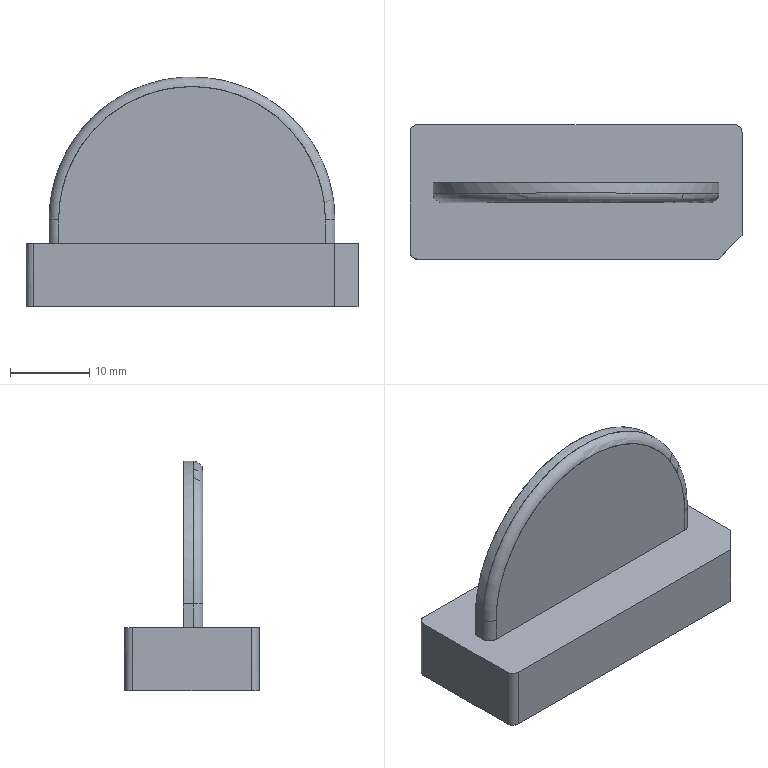NC program | PowerMill | posted with a generic post | part box 42 x 17 x 29.081 mm
Lines 1 to 998 of 145628:
%
O0001
N104 ( POWERMILL CB  : 2026004.0)
N105 ( POST VER      : 2026.0.0.5161)
N106 ( OPTION FILE   : FANUC)
N107 ( OUTPUT WORKPLANE : WORLD)
N108 (  )
N109 ( TOOL LIST )
N110 (---------------------------------------)
N111 ( NO. | ID        | DIA.| TIP RAD|LENGTH)
N112 (---------------------------------------)
N113 (    1|D10C_1_1_1 |10.0 |  0.0   |84.52 )
N114 (    2|D4C_1_1    | 4.0 |  0.0   |76.08 )
N115 (    3|D10_1_1_1  |10.0 |  0.0   |84.24 )
N116 (    7|R2_1_1     | 4.0 |  2.0   | 75.4 )
N117 (   14|D4_1_1     | 4.0 |  0.0   |76.36 )
N118 (   13|TEXT_D4_1_1| 4.0 |  0.3   |76.36 )
N119 (---------------------------------------)
N120 (  )
N121 ( NUMBER OF TOOLPATHS: 10.0 )
N122 ( ESTIMATED PROGRAM DURATION: 0 HOURS 22 MIN 21 SEC)
N123 (  )
N124 G00 G21 G80 G40 G17
N125 G90
N126 G54
N127 G53 Z0.0
N128 (---------------)
N129 ( START TOOLPATH : 精公开粗01-扫面平行-D10C )
N130 (---------------)
N131 ( TOOL NO.    :1 )
N132 ( TOOL TYPE   : ENDMILL)
N133 ( TOOL ID     : D10C_1_1_1)
N134 ( TOOL DIA    : 10.0 LENGTH 84.52)
N135 T1
N136 M6
N137 S8000 M03
N138 G00 G90 X0.0 Y0.0
N139 G43 Z10.2 H1
N140
N141 G05 P10000 R4
N142 X28.78 Y11.28
N143 Z1.128
N144 G01 Z-0.072 F6000.0
N145 X23.78 F10000.0
N146 X-23.78
N147 Y5.64
N148 X23.78
N149 Y0.0
N150 X-23.78
N151 Y-5.64
N152 X23.78
N153 Y-11.28
N154 X-23.78
N155 X-28.78
N156 G00 Z10.2
N157 G05 P0
N158 (---------------)
N159 ( END TOOLPATH : 精公开粗01-扫面平行-D10C )
N160 (---------------)
N161 ( START TOOLPATH : 精公开粗01-外形偏置-D10C )
N162 (---------------)
N163 G00 X-0.0005 Y0.0 Z9.878
N164 G05 P10000 R4
N165 X-4.748 Y16.555
N166 Z0.6824
N167 G01 Z-0.5176 F6000.0
N168 Y16.0275 F10000.0
N169 G03 X-0.0005 Y11.28 I4.7475 J0.0
N170 G01 X24.86
N171 G02 X25.86 Y10.28 I0.0 J-1.0
N172 G01 Y-10.28
N173 G02 X24.86 Y-11.28 I-1.0 J0.0
N174 G01 X-24.861
N175 G02 X-25.861 Y-10.28 I0.0 J1.0
N176 G01 Y10.28
N177 G02 X-24.861 Y11.28 I1.0 J0.0
N178 G01 X-0.0005
N179 Y6.4169
N180 X3.0932 Y6.4168
N181 X3.8666 Y6.399
N182 X4.6401 Y6.3013
N183 X5.4135 Y6.092
N184 X6.0959 Y5.8007
N185 X6.9603 Y5.248
N186 X7.2226 Y5.0273
N187 X7.7338 Y4.5003
N188 X7.9275 Y4.2538
N189 X8.4055 Y3.4804
N190 X8.7187 Y2.707
N191 X8.8992 Y1.9336
N192 X8.9604 Y1.1601
N193 X8.9637 Y-0.3867
N194 X8.9175 Y-0.7813
N195 X14.4064 Y-1.5077
N196 X14.4426 Y-1.2341
N197 G03 X14.5447 Y0.9936 I-12.9021 J1.7075
N198 G01 X14.4426 Y3.5466
N199 G02 X16.748 Y5.6029 I1.9984 J0.08
N200 G01 X18.2762 Y5.3655
N201 G02 X19.9692 Y3.3892 I-0.307 J-1.9763
N202 G01 Y-3.3892
N203 G02 X18.2883 Y-5.3636 I-2.0 J0.0
N204 G01 X16.4548 Y-5.6599
N205 G02 X14.1529 Y-3.4232 I-0.3192 J1.9743
N206 G01 X14.4064 Y-1.5077
N207 X8.9175 Y-0.7813
N208 X8.8732 Y-1.1601
N209 X8.6608 Y-1.9336
N210 X8.3269 Y-2.707
N211 X7.8601 Y-3.4804
N212 X7.7338 Y-3.6456
N213 X7.1694 Y-4.2538
N214 X6.9603 Y-4.4341
N215 X6.1869 Y-4.9724
N216 X5.4135 Y-5.3841
N217 X4.2469 Y-5.8007
N218 X3.8666 Y-5.9112
N219 X3.0932 Y-6.0572
N220 X2.3198 Y-6.1645
N221 X0.7729 Y-6.2839
N222 X-0.7739 Y-6.2838
N223 X-2.3208 Y-6.1644
N224 X-3.0942 Y-6.0571
N225 X-3.8676 Y-5.911
N226 X-4.2415 Y-5.8007
N227 X-5.4145 Y-5.3836
N228 X-6.0923 Y-5.0273
N229 X-6.9613 Y-4.4332
N230 X-7.1687 Y-4.2538
N231 X-7.7348 Y-3.6443
N232 X-7.8604 Y-3.4804
N233 X-8.3275 Y-2.707
N234 X-8.6608 Y-1.9336
N235 X-8.8732 Y-1.1601
N236 X-8.8858 Y-1.0529
N237 X-14.3677 Y-1.7757
N238 X-14.1505 Y-3.4225
N239 G02 X-16.4503 Y-5.6587 I-1.9829 J-0.2614
N240 G01 X-18.2871 Y-5.3639
N241 G02 X-19.9702 Y-3.3892 I0.3169 J1.9747
N242 G01 Y3.3892
N243 G02 X-18.3054 Y5.3609 I2.0 J0.0
N244 G01 X-16.8126 Y5.6146
N245 G02 X-14.4781 Y3.5924 I0.3351 J-1.9717
N246 G01 X-14.5483 Y0.8173
N247 G03 X-14.44 Y-1.2268 I13.0978 J-0.3313
N248 G01 X-14.3677 Y-1.7757
N249 X-8.8858 Y-1.0529
N250 X-8.9637 Y-0.3867
N251 X-8.9611 Y1.1601
N252 X-8.9 Y1.9336
N253 X-8.7217 Y2.707
N254 X-8.4055 Y3.4804
N255 X-7.9294 Y4.2538
N256 X-7.7348 Y4.4991
N257 X-7.2239 Y5.0273
N258 X-6.9613 Y5.2472
N259 X-6.1879 Y5.7527
N260 X-5.4145 Y6.0917
N261 X-4.6411 Y6.3012
N262 X-3.8676 Y6.3989
N263 X-3.0942 Y6.4169
N264 X-0.0005
N265 Y11.28
N266 G00 Z3.2868
N267 G01 X-4.748 Y16.555
N268 G00 Z0.2868
N269 G01 Z-0.9132 F6000.0
N270 Y16.0275 F10000.0
N271 G03 X-0.0005 Y11.28 I4.7475 J0.0
N272 G01 X24.86
N273 G02 X25.86 Y10.28 I0.0 J-1.0
N274 G01 Y-10.28
N275 G02 X24.86 Y-11.28 I-1.0 J0.0
N276 G01 X1.6308
N277 X1.5464 Y-6.5239
N278 X-0.0005 Y-6.5514
N279 X-1.5474 Y-6.5239
N280 X-3.0942 Y-6.4283
N281 X-4.6411 Y-6.2118
N282 X-5.4145 Y-6.0286
N283 X-6.1879 Y-5.8046
N284 X-6.9613 Y-5.4754
N285 X-7.7663 Y-5.0273
N286 X-8.5082 Y-4.4458
N287 X-8.7163 Y-4.2538
N288 X-9.4061 Y-3.4804
N289 X-9.8711 Y-2.707
N290 X-10.1967 Y-1.9336
N291 X-10.3646 Y-1.3222
N292 X-15.8819 Y-2.0602
N293 X-15.6998 Y-3.4218
N294 G02 X-19.1197 Y-5.0774 I-1.9824 J-0.2651
N295 G01 X-19.4077 Y-4.7797
N296 G02 X-19.9702 Y-3.3949 I1.4375 J1.3905
N297 G01 X-19.9901 Y3.6217
N298 G02 X-17.9524 Y5.6271 I2.0 J0.0057
N299 G02 X-15.9917 Y3.5464 I-0.0377 J-1.9997
N300 G01 X-16.095 Y1.0006
N301 G03 X-15.9912 Y-1.2433 I12.9526 J-0.5253
N302 G01 X-15.8819 Y-2.0602
N303 X-10.3646 Y-1.3222
N304 X-10.4092 Y-1.1601
N305 X-10.4958 Y-0.3867
N306 X-10.4842 Y0.3867
N307 X-10.5041 Y1.1601
N308 X-10.4473 Y1.9336
N309 X-10.2658 Y2.707
N310 X-9.954 Y3.4804
N311 X-9.4782 Y4.2538
N312 X-9.2816 Y4.5006
N313 X-8.7737 Y5.0273
N314 X-8.5082 Y5.2463
N315 X-7.7348 Y5.7549
N316 X-6.9613 Y6.0949
N317 X-6.1879 Y6.3042
N318 X-5.4145 Y6.4037
N319 X-4.6411 Y6.4168
N320 X-3.0953
N321 X-3.0942
N322 X-0.454
N323 X4.6401
N324 X5.4135 Y6.4037
N325 X6.1869 Y6.3042
N326 X6.9603 Y6.0953
N327 X7.6483 Y5.8007
N328 X8.5072 Y5.2471
N329 X8.7731 Y5.0273
N330 X9.2806 Y4.5022
N331 X9.4777 Y4.2538
N332 X9.9534 Y3.4804
N333 X10.268 Y2.707
N334 X10.4355 Y1.9892
N335 X16.0291 Y2.2327
N336 X15.9727 Y3.5286
N337 G02 X17.9275 Y5.6152 I1.9981 J0.0871
N338 G02 X19.9708 Y3.6152 I0.0433 J-1.9995
N339 G01 X19.9692 Y-3.3896
N340 G02 X19.426 Y-4.7594 I-2.0 J0.0004
N341 G01 X19.1441 Y-5.0592
N342 G02 X15.7045 Y-3.4271 I-1.4568 J1.3703
N343 G01 X15.9883 Y-1.2779
N344 G03 X16.0856 Y0.9368 I-12.5877 J1.6623
N345 G01 X16.0291 Y2.2327
N346 X10.4355 Y1.9892
N347 X10.4485 Y1.9336
N348 X10.5096 Y1.1601
N349 X10.4844 Y0.3867
N350 X10.4846 Y0.3741
N351 X10.4984 Y-0.3867
N352 X10.4091 Y-1.1601
N353 X10.1957 Y-1.9336
N354 X9.8723 Y-2.707
N355 X9.4032 Y-3.4804
N356 X8.7151 Y-4.2538
N357 X8.5072 Y-4.4467
N358 X7.7661 Y-5.0273
N359 X6.9603 Y-5.4759
N360 X6.2009 Y-5.8007
N361 X5.4135 Y-6.0289
N362 X4.6401 Y-6.212
N363 X3.0932 Y-6.4283
N364 X1.5464 Y-6.5239
N365 X1.6308 Y-11.28
N366 X-24.861
N367 G02 X-25.861 Y-10.28 I0.0 J1.0
N368 G01 Y10.28
N369 G02 X-24.861 Y11.28 I1.0 J0.0
N370 G01 X-0.0005
N371 G00 Z2.8911
N372 G01 X-4.748 Y16.555
N373 G00 Z-0.1089
N374 G01 Z-1.3089 F6000.0
N375 Y16.0275 F10000.0
N376 G03 X-0.0005 Y11.28 I4.7475 J0.0
N377 G01 X24.86
N378 G02 X25.86 Y10.28 I0.0 J-1.0
N379 G01 Y-0.0376
N380 X20.276 Y0.0037
N381 X20.2473 Y-3.8741
N382 G02 X18.4916 Y-5.5316 I-1.6719 J0.0124
N383 G02 X16.9106 Y-3.7066 I0.0838 J1.6699
N384 G01 X17.1834 Y-0.7784
N385 G03 X17.1729 Y1.8028 I-13.2777 J1.2368
N386 G01 X16.9842 Y3.6645
N387 G02 X17.6255 Y4.9931 I1.4025 J0.1422
N388 G01 X17.932 Y5.1897
N389 G02 X20.3047 Y3.8814 I0.8319 J-1.2969
N390 G01 X20.276 Y0.0037
N391 X25.86 Y-0.0376
N392 Y-10.28
N393 G02 X24.86 Y-11.28 I-1.0 J0.0
N394 G01 X1.9457
N395 X1.7958 Y-6.6304
N396 X1.5464 Y-6.6384
N397 X-2.3208 Y-6.6259
N398 X-3.8676 Y-6.5553
N399 X-5.4145 Y-6.3754
N400 X-6.1879 Y-6.2106
N401 X-6.9613 Y-6.0057
N402 X-7.5259 Y-5.8007
N403 X-8.5082 Y-5.3279
N404 X-9.2816 Y-4.8217
N405 X-9.9246 Y-4.2538
N406 X-10.5863 Y-3.4804
N407 X-10.8285 Y-3.1157
N408 X-11.0524 Y-2.707
N409 X-11.3596 Y-1.9336
N410 X-11.57 Y-1.1601
N411 X-11.6598 Y-0.3867
N412 X-11.6619 Y1.1601
N413 X-11.6006 Y1.9336
N414 X-11.4218 Y2.707
N415 X-11.1075 Y3.4804
N416 X-10.8285 Y3.972
N417 X-10.632 Y4.2538
N418 X-10.055 Y4.9096
N419 X-9.2816 Y5.5284
N420 X-8.8142 Y5.8007
N421 X-8.5082 Y5.9471
N422 X-7.7348 Y6.2184
N423 X-6.9613 Y6.3703
N424 X-6.1879 Y6.4168
N425 X6.1869
N426 X6.9603 Y6.3705
N427 X7.7338 Y6.2193
N428 X8.5072 Y5.9476
N429 X8.8128 Y5.8007
N430 X9.2806 Y5.5277
N431 X9.9301 Y5.0273
N432 X10.632 Y4.2538
N433 X10.8275 Y3.9723
N434 X11.1072 Y3.4804
N435 X11.4211 Y2.707
N436 X11.6013 Y1.9336
N437 X11.6624 Y1.1601
N438 X11.6595 Y-0.3867
N439 X11.5703 Y-1.1601
N440 X11.3589 Y-1.9336
N441 X11.0524 Y-2.707
N442 X10.8275 Y-3.1176
N443 X10.5863 Y-3.4804
N444 X9.9243 Y-4.2538
N445 X9.2806 Y-4.8225
N446 X8.5072 Y-5.3285
N447 X7.7338 Y-5.7153
N448 X6.9603 Y-6.006
N449 X6.1869 Y-6.2108
N450 X5.4135 Y-6.3756
N451 X4.6401 Y-6.4769
N452 X3.5423 Y-6.5741
N453 X1.7958 Y-6.6304
N454 X1.9457 Y-11.28
N455 X-24.861
N456 G02 X-25.861 Y-10.28 I0.0 J1.0
N457 G01 Y-0.0375
N458 X-20.2862 Y0.0035
N459 X-20.3147 Y3.8862
N460 G02 X-17.945 Y5.1964 I1.5407 J0.0114
N461 G01 X-17.6293 Y4.9949
N462 G02 X-16.987 Y3.648 I-0.7584 J-1.1882
N463 G01 X-17.1834 Y1.9149
N464 G03 X-17.0637 Y-1.8414 I12.9517 J-1.4676
N465 G01 X-16.778 Y-3.4433
N466 G02 X-17.0925 Y-4.6773 I-1.5169 J-0.2706
N467 G01 X-17.2809 Y-4.9125
N468 G02 X-20.2576 Y-3.8793 I-1.3048 J1.0455
N469 G01 X-20.2862 Y0.0035
N470 X-25.861 Y-0.0375
N471 Y10.28
N472 G02 X-24.861 Y11.28 I1.0 J0.0
N473 G01 X-0.0005
N474 G00 Z2.4955
N475 G01 X-4.748 Y16.555
N476 G00 Z-0.5045
N477 G01 Z-1.7045 F6000.0
N478 Y16.0275 F10000.0
N479 G03 X-0.0005 Y11.28 I4.7475 J0.0
N480 G01 X24.86
N481 G02 X25.86 Y10.28 I0.0 J-1.0
N482 G01 Y-10.28
N483 G02 X24.86 Y-11.28 I-1.0 J0.0
N484 G01 X4.171
N485 X4.06 Y-6.6312
N486 X3.0932 Y-6.6543
N487 X-3.0942
N488 X-4.6411 Y-6.6173
N489 X-5.4145 Y-6.5549
N490 X-6.1879 Y-6.4616
N491 X-6.9613 Y-6.3203
N492 X-7.7348 Y-6.1167
N493 X-8.5082 Y-5.8507
N494 X-9.2816 Y-5.4811
N495 X-9.9973 Y-5.0273
N496 X-10.8285 Y-4.3444
N497 X-11.5537 Y-3.4804
N498 X-12.0192 Y-2.707
N499 X-12.3227 Y-1.9336
N500 X-12.5179 Y-1.1601
N501 X-12.6081 Y-0.3867
N502 X-12.5915 Y0.3867
N503 X-12.6157 Y1.1601
N504 X-12.5592 Y1.878
N505 X-17.9775 Y2.9102
N506 G03 X-17.8345 Y-2.6932 I12.9773 J-2.4723
N507 G01 X-17.5688 Y-3.7822
N508 G02 X-18.2144 Y-5.0414 I-1.0508 J-0.2564
N509 G01 X-18.6701 Y-5.2256
N510 G02 X-20.2471 Y-4.1712 I-0.4298 J1.0637
N511 G01 X-20.3147 Y4.1962
N512 G02 X-19.0619 Y5.1925 I1.0159 J0.0083
N513 G01 X-18.4908 Y5.0556
N514 G02 X-17.7788 Y3.9535 I-0.2216 J-0.9242
N515 G01 X-17.9775 Y2.9102
N516 X-12.5592 Y1.878
N517 X-12.5548 Y1.9336
N518 X-12.3746 Y2.707
N519 X-12.0616 Y3.4804
N520 X-11.5864 Y4.2538
N521 X-10.8845 Y5.0273
N522 X-10.055 Y5.6404
N523 X-9.7687 Y5.8007
N524 X-9.2816 Y6.0228
N525 X-8.5082 Y6.2663
N526 X-7.7348 Y6.391
N527 X-6.9613 Y6.4169
N528 X6.9603
N529 X7.7338 Y6.3911
N530 X8.5072 Y6.2666
N531 X9.2806 Y6.0234
N532 X9.7687 Y5.8007
N533 X10.054 Y5.641
N534 X10.8275 Y5.0755
N535 X11.5864 Y4.2538
N536 X12.0616 Y3.4804
N537 X12.3746 Y2.707
N538 X12.4755 Y2.2737
N539 X17.9038 Y3.2589
N540 X17.7762 Y3.9616
N541 G02 X18.4913 Y5.0559 I0.9352 J0.1698
N542 G01 X19.0586 Y5.191
N543 G02 X20.3098 Y4.1956 I0.2353 J-0.9884
N544 G01 X20.2525 Y-4.1637
N545 G02 X18.6929 Y-5.2263 I-1.1472 J0.0079
N546 G01 X18.2298 Y-5.0479
N547 G02 X17.5655 Y-3.7917 I0.3888 J1.0093
N548 G01 X17.842 Y-2.6127
N549 G03 X17.9803 Y2.8372 I-13.0422 J3.0578
N550 G01 X17.9038 Y3.2589
N551 X12.4755 Y2.2737
N552 X12.5548 Y1.9336
N553 X12.6157 Y1.1601
N554 X12.5914 Y0.3867
N555 X12.5917 Y0.3735
N556 X12.6081 Y-0.3867
N557 X12.5179 Y-1.1601
N558 X12.3246 Y-1.9336
N559 X12.0192 Y-2.707
N560 X11.6009 Y-3.4099
N561 X10.9186 Y-4.2538
N562 X10.054 Y-4.9862
N563 X9.2806 Y-5.4817
N564 X8.6222 Y-5.8007
N565 X7.7338 Y-6.117
N566 X6.9603 Y-6.3205
N567 X6.1869 Y-6.4618
N568 X5.1898 Y-6.5741
N569 X4.6401 Y-6.6174
N570 X4.06 Y-6.6312
N571 X4.171 Y-11.28
N572 X-24.861
N573 G02 X-25.861 Y-10.28 I0.0 J1.0
N574 G01 Y10.28
N575 G02 X-24.861 Y11.28 I1.0 J0.0
N576 G01 X-0.0005
N577 G00 Z2.0999
N578 G01 X-4.748 Y16.555
N579 G00 Z-0.9001
N580 G01 Z-2.1001 F6000.0
N581 Y16.0275 F10000.0
N582 G03 X-0.0005 Y11.28 I4.7475 J0.0
N583 G01 X24.86
N584 G02 X25.86 Y10.28 I0.0 J-1.0
N585 G01 Y-10.28
N586 G02 X24.86 Y-11.28 I-1.0 J0.0
N587 G01 X5.0071
N588 X4.8334 Y-6.647
N589 X4.6401 Y-6.6543
N590 X-4.6411
N591 X-6.1879 Y-6.5962
N592 X-6.9613 Y-6.5145
N593 X-7.7348 Y-6.3715
N594 X-8.5082 Y-6.1769
N595 X-9.2816 Y-5.9168
N596 X-10.055 Y-5.545
N597 X-10.8864 Y-5.0273
N598 X-11.7725 Y-4.2538
N599 X-12.3753 Y-3.4949
N600 X-12.8498 Y-2.707
N601 X-13.155 Y-1.9336
N602 X-13.3428 Y-1.1601
N603 X-13.4339 Y-0.3867
N604 X-13.4319 Y1.1601
N605 X-13.3703 Y1.9336
N606 X-13.1917 Y2.707
N607 X-12.8775 Y3.4804
N608 X-12.403 Y4.2538
N609 X-11.7023 Y5.0273
N610 X-10.8285 Y5.6672
N611 X-10.5893 Y5.8007
N612 X-10.055 Y6.0427
N613 X-9.2816 Y6.279
N614 X-8.5082 Y6.3978
N615 X-7.7348 Y6.4169
N616 X7.7338 Y6.4168
N617 X8.5072 Y6.3979
N618 X9.2806 Y6.2782
N619 X10.054 Y6.0419
N620 X10.5896 Y5.8007
N621 X10.8275 Y5.668
N622 X11.6009 Y5.1148
N623 X12.3743 Y4.292
N624 X12.8775 Y3.4804
N625 X13.1477 Y2.8321
N626 X13.3209 Y2.1326
N627 X19.0523 Y3.2808
N628 X18.7789 Y4.6456
N629 G02 X19.3181 Y5.3716 I0.5973 J0.1197
N630 G02 X19.9853 Y4.7611 I0.0581 J-0.6063
N631 G01 X19.9221 Y-4.5604
N632 X19.9147 Y-4.6628
N633 X19.8941 Y-4.7635
N634 X19.8548 Y-4.9063
N635 G02 X18.9354 Y-5.4138 I-0.7069 J0.1942
N636 G02 X18.452 Y-4.4815 I0.2125 J0.7016
N637 G01 X18.6616 Y-3.8491
N638 G03 X19.2578 Y-0.7416 I-11.5446 J3.8261
N639 G01 X19.2667 Y-0.5927
N640 X19.2905 Y0.075
N641 X19.2829 Y0.7432
N642 X19.255 Y1.5452
N643 G03 X19.0523 Y3.2808 I-10.7315 J-0.3736
N644 G01 X13.3209 Y2.1326
N645 X13.3702 Y1.9336
N646 X13.4311 Y1.1601
N647 X13.4356 Y-0.3867
N648 X13.3455 Y-1.1601
N649 X13.1538 Y-1.9336
N650 X12.8498 Y-2.707
N651 X12.3866 Y-3.4804
N652 X11.7732 Y-4.2538
N653 X10.8863 Y-5.0273
N654 X10.054 Y-5.5455
N655 X9.5583 Y-5.8007
N656 X9.2806 Y-5.9172
N657 X8.5072 Y-6.1773
N658 X7.7338 Y-6.3717
N659 X6.9603 Y-6.5147
N660 X6.4087 Y-6.5741
N661 X6.1869 Y-6.5963
N662 X4.8334 Y-6.647
N663 X5.0071 Y-11.28
N664 X-24.861
N665 G02 X-25.861 Y-10.28 I0.0 J1.0
N666 G01 Y-0.0035
N667 X-19.9717 Y0.0617
N668 X-20.0235 Y4.7512
N669 G02 X-19.3324 Y5.3838 I0.6289 J0.0067
N670 G02 X-18.7794 Y4.6274 I-0.0622 J-0.6259
N671 G01 X-19.057 Y3.3184
N672 G03 X-19.3033 Y0.3163 I11.615 J-2.4638
N673 G01 X-19.2608 Y-0.6189
N674 G03 X-18.6134 Y-3.9841 I11.871 J0.5388
N675 G01 X-18.447 Y-4.4626
N676 G02 X-18.9302 Y-5.4132 I-0.6986 J-0.243
N677 G02 X-19.8611 Y-4.8932 I-0.2154 J0.7076
N678 G01 X-19.8974 Y-4.7546
N679 X-19.9198 Y-4.6278
N680 X-19.9717 Y0.0617
N681 X-25.861 Y-0.0035
N682 Y10.28
N683 G02 X-24.861 Y11.28 I1.0 J0.0
N684 G01 X-0.0005
N685 G00 Z1.7043
N686 G01 X-4.748 Y16.555
N687 G00 Z-1.2957
N688 G01 Z-2.4957 F6000.0
N689 Y16.0275 F10000.0
N690 G03 X-0.0005 Y11.28 I4.7475 J0.0
N691 G01 X19.6402
N692 Y5.4448
N693 G02 X19.9506 Y5.1344 I0.0 J-0.3104
N694 G02 X19.3299 I-0.3104 J0.0
N695 G02 X19.6402 Y5.4448 I0.3103 J0.0
N696 G01 Y11.28
N697 X24.86
N698 G02 X25.86 Y10.28 I0.0 J-1.0
N699 G01 Y-10.28
N700 G02 X24.86 Y-11.28 I-1.0 J0.0
N701 G01 X19.4911
N702 Y-5.5455
N703 G02 X19.0443 Y-5.0988 I0.0 J0.4467
N704 G02 X19.9378 I0.4468 J0.0
N705 G02 X19.4911 Y-5.5455 I-0.4467 J0.0
N706 G01 Y-11.28
N707 X7.0684
N708 X6.9603 Y-6.6184
N709 X5.4135 Y-6.6543
N710 X-4.6411
N711 X-6.1879 Y-6.6503
N712 X-6.9613 Y-6.6184
N713 X-7.4068 Y-6.5741
N714 X-8.5082 Y-6.4004
N715 X-9.2816 Y-6.2054
N716 X-10.3621 Y-5.8007
N717 X-10.8285 Y-5.5615
N718 X-11.6019 Y-5.0755
N719 X-12.5277 Y-4.2538
N720 X-13.1365 Y-3.4804
N721 X-13.5862 Y-2.707
N722 X-13.8918 Y-1.9336
N723 X-14.0837 Y-1.1601
N724 X-14.1739 Y-0.3867
N725 X-14.1743 Y1.1601
N726 X-14.1128 Y1.9336
N727 X-13.9323 Y2.707
N728 X-13.6203 Y3.4804
N729 X-13.1456 Y4.2538
N730 X-12.4458 Y5.0273
N731 X-11.6019 Y5.651
N732 X-11.3353 Y5.8007
N733 X-10.8285 Y6.0314
N734 X-10.055 Y6.2731
N735 X-9.2816 Y6.3952
N736 X-8.5082 Y6.4168
N737 X-7.7354
N738 X-7.7348
N739 X-4.938
N740 X8.5072 Y6.4169
N741 X9.2806 Y6.3951
N742 X10.054 Y6.2734
N743 X10.8275 Y6.0317
N744 X11.3354 Y5.8007
N745 X11.6009 Y5.6516
N746 X12.3743 Y5.0883
N747 X13.1477 Y4.2479
N748 X13.6197 Y3.4804
N749 X13.9323 Y2.707
N750 X14.1123 Y1.9336
N751 X14.1732 Y1.1601
N752 X14.1736 Y-0.3867
N753 X14.0818 Y-1.1601
N754 X13.9212 Y-1.8313
N755 X13.5859 Y-2.707
N756 X13.1477 Y-3.4649
N757 X12.5268 Y-4.2538
N758 X11.6679 Y-5.0273
N759 X10.8275 Y-5.562
N760 X10.3636 Y-5.8007
N761 X9.2806 Y-6.2057
N762 X8.5072 Y-6.4007
N763 X7.4077 Y-6.5741
N764 X6.9603 Y-6.6184
N765 X7.0684 Y-11.28
N766 X-19.5058
N767 Y-5.4105
N768 G02 X-19.8644 Y-5.052 I0.0 J0.3586
N769 G02 X-19.1473 I0.3586 J0.0
N770 G02 X-19.5058 Y-5.4105 I-0.3585 J0.0
N771 G01 Y-11.28
N772 X-24.861
N773 G02 X-25.861 Y-10.28 I0.0 J1.0
N774 G01 Y10.28
N775 G02 X-24.861 Y11.28 I1.0 J0.0
N776 G01 X-19.6505
N777 Y5.4437
N778 G02 X-19.3825 Y5.1757 I0.0 J-0.268
N779 G02 X-19.9186 I-0.268 J0.0
N780 G02 X-19.6505 Y5.4437 I0.2681 J0.0
N781 G01 Y11.28
N782 X-0.0005
N783 G00 Z1.3087
N784 G01 X-4.748 Y16.555
N785 G00 Z-1.6913
N786 G01 Z-2.8914 F6000.0
N787 Y16.0275 F10000.0
N788 G03 X-0.0005 Y11.28 I4.7475 J0.0
N789 G01 X24.86
N790 G02 X25.86 Y10.28 I0.0 J-1.0
N791 G01 Y0.0
N792 X20.3681
N793 Y-5.7319
N794 X20.3517 Y-5.7717
N795 X20.3119 Y-5.7881
N796 X18.8817 Y-5.7882
N797 X18.8527 Y-5.7713
N798 X18.8531 Y-5.7377
N799 X18.8787 Y-5.6951
N800 X19.0663 Y-5.3641
N801 X19.2365 Y-5.0239
N802 X19.2638 Y-4.9654
N803 G03 X20.1343 Y-2.2039 I-9.9333 J4.649
N804 G01 X20.1504 Y-2.1114
N805 G03 X20.3279 Y-0.0144 I-11.7255 J2.0486
N806 G01 X20.3266 Y0.3172
N807 X20.3322 Y0.8642
N808 X20.3328 Y1.0232
N809 X20.3314 Y1.1821
N810 X20.3294 Y1.3097
N811 X20.3155 Y1.7111
N812 X20.2866 Y2.1117
N813 X20.2858 Y2.1203
N814 G03 X19.3282 Y5.6625 I-10.6085 J-0.9674
N815 G01 X19.2933 Y5.7371
N816 X19.2956 Y5.7715
N817 X19.3259 Y5.7882
N818 X20.3119 Y5.7881
N819 X20.3517 Y5.7717
N820 X20.3681 Y5.7319
N821 Y0.0
N822 X25.86
N823 Y-10.28
N824 G02 X24.86 Y-11.28 I-1.0 J0.0
N825 G01 X7.9154
N826 X7.7338 Y-6.624
N827 X6.9603 Y-6.6542
N828 X5.4151
N829 X5.4135
N830 X-4.6411
N831 X-4.6574
N832 X-6.9613
N833 X-7.7348 Y-6.624
N834 X-8.2636 Y-6.5741
N835 X-9.2816 Y-6.4085
N836 X-10.055 Y-6.2003
N837 X-11.0787 Y-5.8007
N838 X-11.6019 Y-5.523
N839 X-12.3753 Y-5.0217
N840 X-13.1488 Y-4.3164
N841 X-13.8212 Y-3.4804
N842 X-14.2573 Y-2.707
N843 X-14.5613 Y-1.9336
N844 X-14.6956 Y-1.3886
N845 X-14.8282 Y-0.3867
N846 X-14.8171 Y0.3867
N847 X-14.8391 Y1.1601
N848 X-14.7782 Y1.9336
N849 X-14.5985 Y2.707
N850 X-14.2865 Y3.4804
N851 X-13.8131 Y4.2538
N852 X-13.1488 Y4.9953
N853 X-12.3753 Y5.5884
N854 X-12.0078 Y5.8007
N855 X-11.6019 Y5.9916
N856 X-10.8285 Y6.2499
N857 X-10.055 Y6.3864
N858 X-9.2816 Y6.4169
N859 X7.1124 Y6.4168
N860 X8.5072
N861 X8.5076
N862 X9.2806
N863 X10.054 Y6.3868
N864 X10.8275 Y6.2508
N865 X11.6009 Y5.9921
N866 X12.0077 Y5.8007
N867 X12.3743 Y5.589
N868 X13.1147 Y5.0273
N869 X13.8131 Y4.2538
N870 X14.2865 Y3.4804
N871 X14.5986 Y2.707
N872 X14.7782 Y1.9336
N873 X14.839 Y1.1601
N874 X14.8171 Y0.3867
N875 X14.8172 Y0.376
N876 X14.8281 Y-0.3867
N877 X14.7385 Y-1.1601
N878 X14.562 Y-1.9336
N879 X14.2573 Y-2.707
N880 X13.8212 Y-3.4804
N881 X13.2115 Y-4.2538
N882 X12.3743 Y-5.0225
N883 X11.6009 Y-5.5236
N884 X11.0757 Y-5.8007
N885 X10.054 Y-6.2006
N886 X9.2806 Y-6.4087
N887 X8.2647 Y-6.5741
N888 X7.7338 Y-6.624
N889 X7.9154 Y-11.28
N890 X-24.861
N891 G02 X-25.861 Y-10.28 I0.0 J1.0
N892 G01 Y0.0
N893 X-20.3692
N894 Y5.7319
N895 X-20.3527 Y5.7717
N896 X-20.3129 Y5.7881
N897 X-19.3259 Y5.7882
N898 X-19.2956 Y5.7715
N899 X-19.2933 Y5.7371
N900 X-19.3287 Y5.6614
N901 G03 X-20.2792 Y2.1894 I9.65 J-4.5079
N902 G01 X-20.2801 Y2.1796
N903 X-20.3138 Y1.742
N904 X-20.3295 Y1.3034
N905 X-20.3314 Y1.1792
N906 X-20.3328 Y1.0227
N907 X-20.3321 Y0.8662
N908 X-20.3265 Y0.3273
N909 X-20.3288 Y0.1863
N910 G03 X-20.1978 Y-1.7814 I11.7112 J-0.2087
N911 G01 X-20.1586 Y-2.0394
N912 G03 X-19.5049 Y-4.3931 I10.0745 J1.5303
N913 G01 X-19.3713 Y-4.7171
N914 X-19.1563 Y-5.1896
N915 X-18.9079 Y-5.6453
N916 X-18.853 Y-5.7379
N917 X-18.8528 Y-5.7714
N918 X-18.8817 Y-5.7882
N919 X-20.3129 Y-5.7881
N920 X-20.3527 Y-5.7717
N921 X-20.3692 Y-5.7319
N922 Y0.0
N923 X-25.861
N924 Y10.28
N925 G02 X-24.861 Y11.28 I1.0 J0.0
N926 G01 X-0.0005
N927 G00 Z0.913
N928 G01 X-4.748 Y16.555
N929 G00 Z-2.087
N930 G01 Z-3.287 F6000.0
N931 Y16.0275 F10000.0
N932 G03 X-0.0005 Y11.28 I4.7475 J0.0
N933 G01 X24.86
N934 G02 X25.86 Y10.28 I0.0 J-1.0
N935 G01 Y0.0
N936 X21.36
N937 Y-6.28
N938 G02 X20.86 Y-6.78 I-0.5 J0.0
N939 G01 X18.5777
N940 G02 X18.1634 Y-6.0 I0.0 J0.5
N941 G01 X18.26 Y-5.8509
N942 X18.3506 Y-5.698
N943 X18.7886 Y-4.9246
N944 X18.9342 Y-4.645
N945 X19.0599 Y-4.356
N946 X19.3645 Y-3.5826
N947 X19.4785 Y-3.2572
N948 X19.5672 Y-2.9241
N949 X19.7417 Y-2.1507
N950 X19.7875 Y-1.9199
N951 X19.8211 Y-1.687
N952 X19.9123 Y-0.9135
N953 X19.9356 Y-0.6497
N954 X19.9433 Y-0.385
N955 X19.9427 Y1.1619
N956 X19.9392 Y1.3376
N957 X19.9288 Y1.513
N958 X19.868 Y2.2864
N959 X19.829 Y2.6212
N960 X19.7651 Y2.952
N961 X19.5854 Y3.7255
N962 X19.493 Y4.0629
N963 X19.3747 Y4.3922
N964 X19.0623 Y5.1656
N965 X18.9518 Y5.4169
N966 X18.8262 Y5.661
N967 X18.631 Y6.0133
N968 X18.6249 Y6.0243
N969 X18.6187 Y6.0353
N970 G02 X19.0547 Y6.78 I0.436 J0.2447
N971 G01 X20.86
N972 G02 X21.36 Y6.28 I0.0 J-0.5
N973 G01 Y0.0
N974 X25.86
N975 Y-10.28
N976 G02 X24.86 Y-11.28 I-1.0 J0.0
N977 G01 X-0.0005
N978 Y-6.6543
N979 X-7.7348
N980 X-8.5082 Y-6.6239
N981 X-9.0242 Y-6.5741
N982 X-10.055 Y-6.3917
N983 X-10.8285 Y-6.1726
N984 X-11.6019 Y-5.8571
N985 X-12.3753 Y-5.4434
N986 X-13.1488 Y-4.9006
N987 X-13.8271 Y-4.2538
N988 X-14.4358 Y-3.4804
N989 X-14.873 Y-2.707
N990 X-15.1751 Y-1.9336
N991 X-15.3541 Y-1.1601
N992 X-15.4426 Y-0.3867
N993 X-15.4427 Y1.1601
N994 X-15.3822 Y1.9336
N995 X-15.2 Y2.707
N996 X-14.8903 Y3.4804
N997 X-14.6956 Y3.831
N998 X-14.4167 Y4.2538
N999 X-13.9222 Y4.8301
N1000 X-13.718 Y5.0273
N1001 X-13.1488 Y5.4764
N1002 X-12.6106 Y5.8007
N1003 X-12.3753 Y5.9154
N1004 X-11.6019 Y6.2031
N1005 X-10.8285 Y6.3666
N1006 X-10.055 Y6.4168
N1007 X-9.2826
N1008 X-9.2816
N1009 X-3.7986
N1010 X10.054 Y6.4169
N1011 X10.8275 Y6.3668
N1012 X11.6009 Y6.2034
N1013 X12.3743 Y5.9159
N1014 X12.61 Y5.8007
N1015 X13.1477 Y5.4771
N1016 X13.7179 Y5.0273
N1017 X13.9212 Y4.8307
N1018 X14.4159 Y4.2538
N1019 X14.6946 Y3.8327
N1020 X14.8898 Y3.4804
N1021 X15.2021 Y2.707
N1022 X15.3818 Y1.9336
N1023 X15.4427 Y1.1601
N1024 X15.4433 Y-0.3867
N1025 X15.3521 Y-1.1601
N1026 X15.1776 Y-1.9336
N1027 X14.873 Y-2.707
N1028 X14.4349 Y-3.4804
N1029 X13.9212 Y-4.1499
N1030 X13.1477 Y-4.9014
N1031 X12.3743 Y-5.4441
N1032 X11.729 Y-5.8007
N1033 X10.8275 Y-6.173
N1034 X10.054 Y-6.392
N1035 X9.0252 Y-6.5741
N1036 X8.5072 Y-6.624
N1037 X7.7338 Y-6.6543
N1038 X-0.0005
N1039 Y-11.28
N1040 X-24.861
N1041 G02 X-25.861 Y-10.28 I0.0 J1.0
N1042 G01 Y0.0
N1043 X-21.361
N1044 Y6.28
N1045 G02 X-20.861 Y6.78 I0.5 J0.0
N1046 G01 X-19.0548
N1047 G02 X-18.6189 Y6.0351 I0.0 J-0.5
N1048 G01 X-18.6243 Y6.0255
N1049 X-18.6297 Y6.0158
N1050 X-18.8244 Y5.6652
N1051 X-18.9542 Y5.413
N1052 X-19.0678 Y5.1532
N1053 X-19.3775 Y4.3798
N1054 X-19.4909 Y4.0629
N1055 X-19.5802 Y3.7385
N1056 X-19.7624 Y2.965
N1057 X-19.8284 Y2.6268
N1058 X-19.8685 Y2.2845
N1059 X-19.929 Y1.5111
N1060 X-19.9392 Y1.3357
N1061 X-19.9427 Y1.16
N1062 X-19.9426 Y-0.3869
N1063 X-19.9353 Y-0.643
N1064 X-19.9134 Y-0.8983
N1065 X-19.8249 Y-1.6717
N1066 X-19.7887 Y-1.9244
N1067 X-19.7383 Y-2.1747
N1068 X-19.5593 Y-2.9481
N1069 X-19.4742 Y-3.2631
N1070 X-19.3666 Y-3.5712
N1071 X-19.0644 Y-4.3446
N1072 X-18.9376 Y-4.6379
N1073 X-18.7904 Y-4.9214
N1074 X-18.3532 Y-5.6948
N1075 X-18.2618 Y-5.8493
N1076 X-18.1642 Y-6.0
N1077 G02 X-18.5785 Y-6.78 I-0.4143 J-0.28
N1078 G01 X-20.861
N1079 G02 X-21.361 Y-6.28 I0.0 J0.5
N1080 G01 Y0.0
N1081 X-25.861
N1082 Y10.28
N1083 G02 X-24.861 Y11.28 I1.0 J0.0
N1084 G01 X-0.0005
N1085 G00 Z0.5174
N1086 G01 X-4.748 Y16.555
N1087 G00 Z-2.4826
N1088 G01 Z-3.6826 F6000.0
N1089 Y16.0275 F10000.0
N1090 G03 X-0.0005 Y11.28 I4.7475 J0.0
N1091 G01 X24.86
N1092 G02 X25.86 Y10.28 I0.0 J-1.0
N1093 G01 Y4.5275
N1094 X21.36
N1095 X25.86